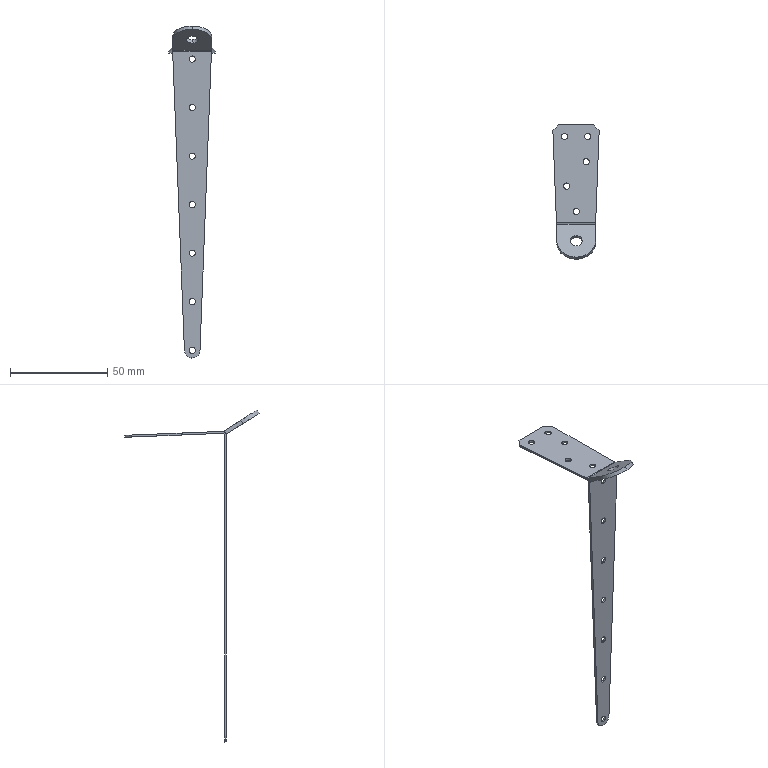Part | SolidWorks | features BaseBody 2 | 2 solids | 51 faces | box 23.767 x 69.031 x 170.393 mm | volume 3866 mm3 | cylinder 33 | plane 16 | spline 2 | commonest cylinder face diameters 3.2 x24 2 x2 4 x2 6.35 x2 20 x2 8 x1